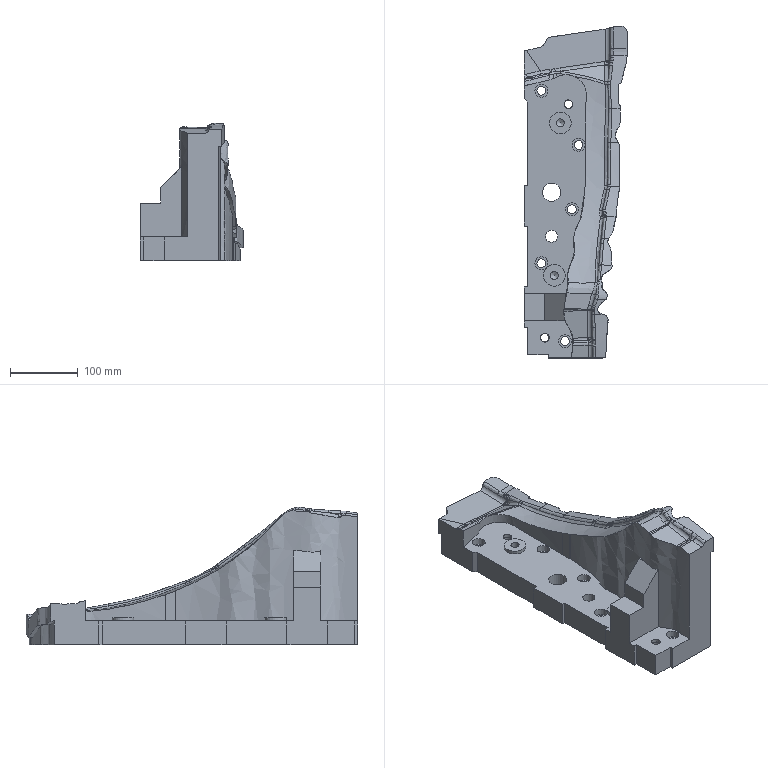Part | NX | features solid 2 | 1 solid | 217 faces | box 152.31 x 490.732 x 202.902 mm | volume 4159925 mm3 | spline 118 | plane 54 | cylinder 40 | sphere 3 | cone 2 | commonest cylinder face diameters 12 x11 13 x7 19 x5 10 x2 32 x2 9.966 x1